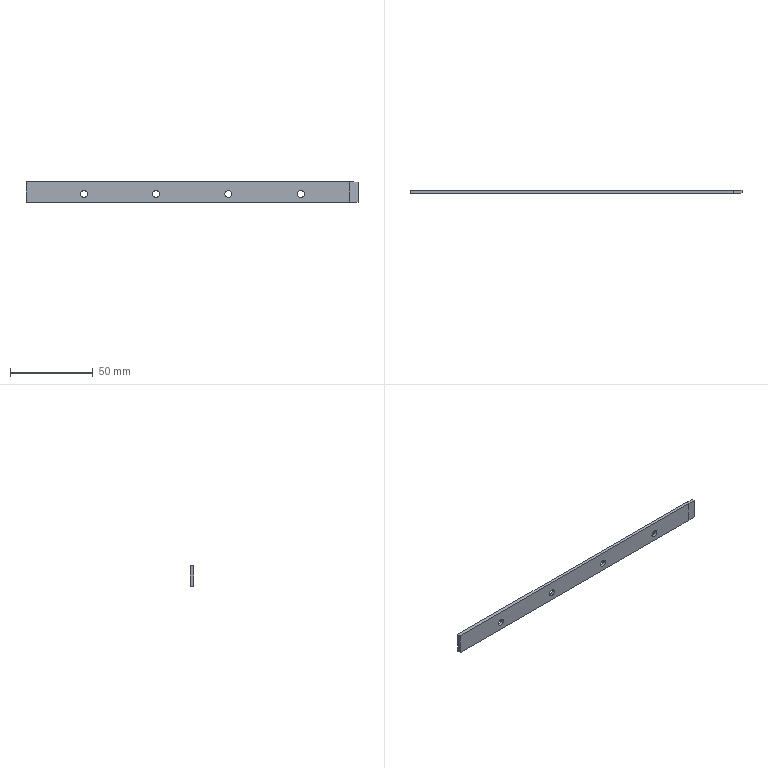Part | NX | 1 solid | 24 faces | box 200 x 2 x 12.5 mm | volume 4873 mm3 | plane 8 | cylinder 8 | cone 8 | commonest cylinder face diameters 4.2 x8
STEP:
#1=CARTESIAN_POINT('',(-140.,215.4,-65.8));
#2=VERTEX_POINT('',#1);
#3=CARTESIAN_POINT('',(-140.,215.4,-53.3));
#4=VERTEX_POINT('',#3);
#5=CARTESIAN_POINT('',(-140.,215.4,-59.293));
#6=DIRECTION('',(0.,0.,1.));
#7=VECTOR('',#6,1000.);
#8=LINE('',#5,#7);
#9=EDGE_CURVE('',#2,#4,#8,.T.);
#10=ORIENTED_EDGE('',*,*,#9,.T.);
#11=CARTESIAN_POINT('',(-140.,217.4,-53.3));
#12=VERTEX_POINT('',#11);
#13=CARTESIAN_POINT('',(-140.,215.4,-53.3));
#14=DIRECTION('',(0.,1.,0.));
#15=VECTOR('',#14,1000.);
#16=LINE('',#13,#15);
#17=EDGE_CURVE('',#4,#12,#16,.T.);
#18=ORIENTED_EDGE('',*,*,#17,.T.);
#19=CARTESIAN_POINT('',(-140.,217.4,-65.8));
#20=VERTEX_POINT('',#19);
#21=CARTESIAN_POINT('',(-140.,217.4,-59.293));
#22=DIRECTION('',(0.,0.,1.));
#23=VECTOR('',#22,1000.);
#24=LINE('',#21,#23);
#25=EDGE_CURVE('',#20,#12,#24,.T.);
#26=ORIENTED_EDGE('',*,*,#25,.F.);
#27=CARTESIAN_POINT('',(-140.,215.4,-65.8));
#28=DIRECTION('',(0.,1.,0.));
#29=VECTOR('',#28,1000.);
#30=LINE('',#27,#29);
#31=EDGE_CURVE('',#2,#20,#30,.T.);
#32=ORIENTED_EDGE('',*,*,#31,.F.);
#33=EDGE_LOOP('',(#10,#18,#26,#32));
#34=FACE_BOUND('',#33,.T.);
#35=CARTESIAN_POINT('',(-140.,215.4,-55.8));
#36=DIRECTION('',(-1.,0.,0.));
#37=DIRECTION('',(0.,0.,1.));
#38=AXIS2_PLACEMENT_3D('',#35,#36,#37);
#39=PLANE('',#38);
#40=ADVANCED_FACE('',(#34),#39,.T.);
#41=CARTESIAN_POINT('',(55.,217.4,-53.3));
#42=VERTEX_POINT('',#41);
#43=CARTESIAN_POINT('',(55.,215.4,-53.3));
#44=VERTEX_POINT('',#43);
#45=CARTESIAN_POINT('',(55.,216.4,-53.3));
#46=DIRECTION('',(0.,-1.,0.));
#47=VECTOR('',#46,1000.);
#48=LINE('',#45,#47);
#49=EDGE_CURVE('',#42,#44,#48,.T.);
#50=ORIENTED_EDGE('',*,*,#49,.F.);
#51=CARTESIAN_POINT('',(-59.483,217.4,-53.3));
#52=DIRECTION('',(1.,0.,0.));
#53=VECTOR('',#52,1000.);
#54=LINE('',#51,#53);
#55=EDGE_CURVE('',#12,#42,#54,.T.);
#56=ORIENTED_EDGE('',*,*,#55,.F.);
#57=ORIENTED_EDGE('',*,*,#17,.F.);
#58=CARTESIAN_POINT('',(-59.483,215.4,-53.3));
#59=DIRECTION('',(1.,0.,0.));
#60=VECTOR('',#59,1000.);
#61=LINE('',#58,#60);
#62=EDGE_CURVE('',#4,#44,#61,.T.);
#63=ORIENTED_EDGE('',*,*,#62,.T.);
#64=EDGE_LOOP('',(#50,#56,#57,#63));
#65=FACE_BOUND('',#64,.T.);
#66=CARTESIAN_POINT('',(60.,215.4,-53.3));
#67=DIRECTION('',(0.,0.,1.));
#68=DIRECTION('',(1.,0.,0.));
#69=AXIS2_PLACEMENT_3D('',#66,#67,#68);
#70=PLANE('',#69);
#71=ADVANCED_FACE('',(#65),#70,.T.);
#72=CARTESIAN_POINT('',(60.,215.837,-53.737));
#73=VERTEX_POINT('',#72);
#74=CARTESIAN_POINT('',(60.,215.837,-65.8));
#75=VERTEX_POINT('',#74);
#76=CARTESIAN_POINT('',(60.,215.837,-59.55));
#77=DIRECTION('',(0.,0.,-1.));
#78=VECTOR('',#77,1000.);
#79=LINE('',#76,#78);
#80=EDGE_CURVE('',#73,#75,#79,.T.);
#81=ORIENTED_EDGE('',*,*,#80,.T.);
#82=CARTESIAN_POINT('',(60.,217.4,-65.8));
#83=VERTEX_POINT('',#82);
#84=CARTESIAN_POINT('',(60.,215.4,-65.8));
#85=DIRECTION('',(0.,1.,0.));
#86=VECTOR('',#85,1000.);
#87=LINE('',#84,#86);
#88=EDGE_CURVE('',#75,#83,#87,.T.);
#89=ORIENTED_EDGE('',*,*,#88,.T.);
#90=CARTESIAN_POINT('',(60.,217.4,-53.737));
#91=VERTEX_POINT('',#90);
#92=CARTESIAN_POINT('',(60.,217.4,-59.293));
#93=DIRECTION('',(0.,0.,-1.));
#94=VECTOR('',#93,1000.);
#95=LINE('',#92,#94);
#96=EDGE_CURVE('',#91,#83,#95,.T.);
#97=ORIENTED_EDGE('',*,*,#96,.F.);
#98=CARTESIAN_POINT('',(60.,216.4,-53.737));
#99=DIRECTION('',(0.,-1.,0.));
#100=VECTOR('',#99,1000.);
#101=LINE('',#98,#100);
#102=EDGE_CURVE('',#91,#73,#101,.T.);
#103=ORIENTED_EDGE('',*,*,#102,.T.);
#104=EDGE_LOOP('',(#81,#89,#97,#103));
#105=FACE_BOUND('',#104,.T.);
#106=CARTESIAN_POINT('',(60.,215.4,-65.8));
#107=DIRECTION('',(1.,0.,0.));
#108=DIRECTION('',(0.,-1.,0.));
#109=AXIS2_PLACEMENT_3D('',#106,#107,#108);
#110=PLANE('',#109);
#111=ADVANCED_FACE('',(#105),#110,.T.);
#112=CARTESIAN_POINT('',(55.,215.4,-65.8));
#113=VERTEX_POINT('',#112);
#114=CARTESIAN_POINT('',(60.,215.4,-65.8));
#115=DIRECTION('',(-1.,0.,0.));
#116=VECTOR('',#115,1000.);
#117=LINE('',#114,#116);
#118=EDGE_CURVE('',#113,#2,#117,.T.);
#119=ORIENTED_EDGE('',*,*,#118,.T.);
#120=ORIENTED_EDGE('',*,*,#31,.T.);
#121=CARTESIAN_POINT('',(60.,217.4,-65.8));
#122=DIRECTION('',(-1.,0.,0.));
#123=VECTOR('',#122,1000.);
#124=LINE('',#121,#123);
#125=EDGE_CURVE('',#83,#20,#124,.T.);
#126=ORIENTED_EDGE('',*,*,#125,.F.);
#127=ORIENTED_EDGE('',*,*,#88,.F.);
#128=CARTESIAN_POINT('',(-59.483,205.384,-65.8));
#129=DIRECTION('',(-0.9962,-0.08716,0.));
#130=VECTOR('',#129,1000.);
#131=LINE('',#128,#130);
#132=EDGE_CURVE('',#75,#113,#131,.T.);
#133=ORIENTED_EDGE('',*,*,#132,.T.);
#134=EDGE_LOOP('',(#119,#120,#126,#127,#133));
#135=FACE_BOUND('',#134,.T.);
#136=CARTESIAN_POINT('',(-140.,215.4,-65.8));
#137=DIRECTION('',(0.,0.,-1.));
#138=DIRECTION('',(0.,-1.,0.));
#139=AXIS2_PLACEMENT_3D('',#136,#137,#138);
#140=PLANE('',#139);
#141=ADVANCED_FACE('',(#135),#140,.T.);
#142=ORIENTED_EDGE('',*,*,#49,.T.);
#143=CARTESIAN_POINT('',(-59.483,205.384,-43.284));
#144=DIRECTION('',(-0.9924,-0.08683,0.08683));
#145=VECTOR('',#144,1000.);
#146=LINE('',#143,#145);
#147=EDGE_CURVE('',#73,#44,#146,.T.);
#148=ORIENTED_EDGE('',*,*,#147,.F.);
#149=ORIENTED_EDGE('',*,*,#102,.F.);
#150=CARTESIAN_POINT('',(-59.483,217.4,-43.284));
#151=DIRECTION('',(0.9962,0.,-0.08716));
#152=VECTOR('',#151,1000.);
#153=LINE('',#150,#152);
#154=EDGE_CURVE('',#42,#91,#153,.T.);
#155=ORIENTED_EDGE('',*,*,#154,.F.);
#156=EDGE_LOOP('',(#142,#148,#149,#155));
#157=FACE_BOUND('',#156,.T.);
#158=CARTESIAN_POINT('',(57.5,216.4,-53.519));
#159=DIRECTION('',(-0.08716,0.,-0.9962));
#160=DIRECTION('',(-0.9962,0.,0.08716));
#161=AXIS2_PLACEMENT_3D('',#158,#159,#160);
#162=PLANE('',#161);
#163=ADVANCED_FACE('',(#157),#162,.F.);
#164=ORIENTED_EDGE('',*,*,#96,.T.);
#165=ORIENTED_EDGE('',*,*,#125,.T.);
#166=ORIENTED_EDGE('',*,*,#25,.T.);
#167=ORIENTED_EDGE('',*,*,#55,.T.);
#168=ORIENTED_EDGE('',*,*,#154,.T.);
#169=EDGE_LOOP('',(#164,#165,#166,#167,#168));
#170=FACE_BOUND('',#169,.T.);
#171=CARTESIAN_POINT('',(27.925,217.4,-60.8));
#172=VERTEX_POINT('',#171);
#173=CARTESIAN_POINT('',(23.325,217.4,-60.8));
#174=VERTEX_POINT('',#173);
#175=CARTESIAN_POINT('',(25.625,217.4,-60.8));
#176=DIRECTION('',(0.,1.,0.));
#177=DIRECTION('',(-1.,0.,0.));
#178=AXIS2_PLACEMENT_3D('',#175,#176,#177);
#179=CIRCLE('',#178,2.3);
#180=EDGE_CURVE('',#172,#174,#179,.T.);
#181=ORIENTED_EDGE('',*,*,#180,.F.);
#182=CARTESIAN_POINT('',(25.625,217.4,-60.8));
#183=DIRECTION('',(0.,1.,0.));
#184=DIRECTION('',(-1.,0.,0.));
#185=AXIS2_PLACEMENT_3D('',#182,#183,#184);
#186=CIRCLE('',#185,2.3);
#187=EDGE_CURVE('',#174,#172,#186,.T.);
#188=ORIENTED_EDGE('',*,*,#187,.F.);
#189=EDGE_LOOP('',(#181,#188));
#190=FACE_BOUND('',#189,.T.);
#191=CARTESIAN_POINT('',(-107.364,217.4,-60.8));
#192=VERTEX_POINT('',#191);
#193=CARTESIAN_POINT('',(-102.764,217.4,-60.8));
#194=VERTEX_POINT('',#193);
#195=CARTESIAN_POINT('',(-105.064,217.4,-60.8));
#196=DIRECTION('',(0.,1.,0.));
#197=DIRECTION('',(-1.,0.,0.));
#198=AXIS2_PLACEMENT_3D('',#195,#196,#197);
#199=CIRCLE('',#198,2.3);
#200=EDGE_CURVE('',#192,#194,#199,.T.);
#201=ORIENTED_EDGE('',*,*,#200,.F.);
#202=CARTESIAN_POINT('',(-105.064,217.4,-60.8));
#203=DIRECTION('',(0.,1.,0.));
#204=DIRECTION('',(-1.,0.,0.));
#205=AXIS2_PLACEMENT_3D('',#202,#203,#204);
#206=CIRCLE('',#205,2.3);
#207=EDGE_CURVE('',#194,#192,#206,.T.);
#208=ORIENTED_EDGE('',*,*,#207,.F.);
#209=EDGE_LOOP('',(#201,#208));
#210=FACE_BOUND('',#209,.T.);
#211=CARTESIAN_POINT('',(-20.425,217.4,-60.8));
#212=VERTEX_POINT('',#211);
#213=CARTESIAN_POINT('',(-15.825,217.4,-60.8));
#214=VERTEX_POINT('',#213);
#215=CARTESIAN_POINT('',(-18.125,217.4,-60.8));
#216=DIRECTION('',(0.,1.,0.));
#217=DIRECTION('',(-1.,0.,0.));
#218=AXIS2_PLACEMENT_3D('',#215,#216,#217);
#219=CIRCLE('',#218,2.3);
#220=EDGE_CURVE('',#212,#214,#219,.T.);
#221=ORIENTED_EDGE('',*,*,#220,.F.);
#222=CARTESIAN_POINT('',(-18.125,217.4,-60.8));
#223=DIRECTION('',(0.,1.,0.));
#224=DIRECTION('',(-1.,0.,0.));
#225=AXIS2_PLACEMENT_3D('',#222,#223,#224);
#226=CIRCLE('',#225,2.3);
#227=EDGE_CURVE('',#214,#212,#226,.T.);
#228=ORIENTED_EDGE('',*,*,#227,.F.);
#229=EDGE_LOOP('',(#221,#228));
#230=FACE_BOUND('',#229,.T.);
#231=CARTESIAN_POINT('',(-59.388,217.4,-60.8));
#232=VERTEX_POINT('',#231);
#233=CARTESIAN_POINT('',(-63.988,217.4,-60.8));
#234=VERTEX_POINT('',#233);
#235=CARTESIAN_POINT('',(-61.688,217.4,-60.8));
#236=DIRECTION('',(0.,1.,0.));
#237=DIRECTION('',(-1.,0.,0.));
#238=AXIS2_PLACEMENT_3D('',#235,#236,#237);
#239=CIRCLE('',#238,2.3);
#240=EDGE_CURVE('',#232,#234,#239,.T.);
#241=ORIENTED_EDGE('',*,*,#240,.F.);
#242=CARTESIAN_POINT('',(-61.688,217.4,-60.8));
#243=DIRECTION('',(0.,1.,0.));
#244=DIRECTION('',(-1.,0.,0.));
#245=AXIS2_PLACEMENT_3D('',#242,#243,#244);
#246=CIRCLE('',#245,2.3);
#247=EDGE_CURVE('',#234,#232,#246,.T.);
#248=ORIENTED_EDGE('',*,*,#247,.F.);
#249=EDGE_LOOP('',(#241,#248));
#250=FACE_BOUND('',#249,.T.);
#251=CARTESIAN_POINT('',(-59.483,217.4,-59.293));
#252=DIRECTION('',(0.,1.,0.));
#253=DIRECTION('',(1.,0.,0.));
#254=AXIS2_PLACEMENT_3D('',#251,#252,#253);
#255=PLANE('',#254);
#256=ADVANCED_FACE('',(#170,#190,#210,#230,#250),#255,.T.);
#257=CARTESIAN_POINT('',(-20.225,215.4,-60.8));
#258=VERTEX_POINT('',#257);
#259=CARTESIAN_POINT('',(-16.025,215.4,-60.8));
#260=VERTEX_POINT('',#259);
#261=CARTESIAN_POINT('',(-18.125,215.4,-60.8));
#262=DIRECTION('',(0.,1.,0.));
#263=DIRECTION('',(-1.,0.,0.));
#264=AXIS2_PLACEMENT_3D('',#261,#262,#263);
#265=CIRCLE('',#264,2.1);
#266=EDGE_CURVE('',#258,#260,#265,.T.);
#267=ORIENTED_EDGE('',*,*,#266,.F.);
#268=CARTESIAN_POINT('',(-20.225,217.2,-60.8));
#269=VERTEX_POINT('',#268);
#270=CARTESIAN_POINT('',(-20.225,217.4,-60.8));
#271=DIRECTION('',(0.,1.,0.));
#272=VECTOR('',#271,1000.);
#273=LINE('',#270,#272);
#274=EDGE_CURVE('',#269,#258,#273,.F.);
#275=ORIENTED_EDGE('',*,*,#274,.F.);
#276=CARTESIAN_POINT('',(-16.025,217.2,-60.8));
#277=VERTEX_POINT('',#276);
#278=CARTESIAN_POINT('',(-18.125,217.2,-60.8));
#279=DIRECTION('',(0.,1.,0.));
#280=DIRECTION('',(-1.,0.,0.));
#281=AXIS2_PLACEMENT_3D('',#278,#279,#280);
#282=CIRCLE('',#281,2.1);
#283=EDGE_CURVE('',#269,#277,#282,.T.);
#284=ORIENTED_EDGE('',*,*,#283,.T.);
#285=CARTESIAN_POINT('',(-16.025,217.4,-60.8));
#286=DIRECTION('',(0.,1.,0.));
#287=VECTOR('',#286,1000.);
#288=LINE('',#285,#287);
#289=EDGE_CURVE('',#277,#260,#288,.F.);
#290=ORIENTED_EDGE('',*,*,#289,.T.);
#291=EDGE_LOOP('',(#267,#275,#284,#290));
#292=FACE_BOUND('',#291,.T.);
#293=CARTESIAN_POINT('',(-18.125,217.4,-60.8));
#294=DIRECTION('',(0.,1.,0.));
#295=DIRECTION('',(-1.,0.,0.));
#296=AXIS2_PLACEMENT_3D('',#293,#294,#295);
#297=CYLINDRICAL_SURFACE('',#296,2.1);
#298=ADVANCED_FACE('',(#292),#297,.F.);
#299=ORIENTED_EDGE('',*,*,#220,.T.);
#300=CARTESIAN_POINT('',(-16.025,217.2,-60.8));
#301=DIRECTION('',(0.7071,0.7071,0.));
#302=VECTOR('',#301,1000.);
#303=LINE('',#300,#302);
#304=EDGE_CURVE('',#277,#214,#303,.T.);
#305=ORIENTED_EDGE('',*,*,#304,.F.);
#306=ORIENTED_EDGE('',*,*,#283,.F.);
#307=CARTESIAN_POINT('',(-20.225,217.2,-60.8));
#308=DIRECTION('',(-0.7071,0.7071,0.));
#309=VECTOR('',#308,1000.);
#310=LINE('',#307,#309);
#311=EDGE_CURVE('',#269,#212,#310,.T.);
#312=ORIENTED_EDGE('',*,*,#311,.T.);
#313=EDGE_LOOP('',(#299,#305,#306,#312));
#314=FACE_BOUND('',#313,.T.);
#315=CARTESIAN_POINT('',(-18.125,217.2,-60.8));
#316=DIRECTION('',(0.,1.,0.));
#317=DIRECTION('',(1.,0.,0.));
#318=AXIS2_PLACEMENT_3D('',#315,#316,#317);
#319=CONICAL_SURFACE('',#318,2.1,0.7854);
#320=ADVANCED_FACE('',(#314),#319,.F.);
#321=CARTESIAN_POINT('',(27.725,215.4,-60.8));
#322=VERTEX_POINT('',#321);
#323=CARTESIAN_POINT('',(23.525,215.4,-60.8));
#324=VERTEX_POINT('',#323);
#325=CARTESIAN_POINT('',(25.625,215.4,-60.8));
#326=DIRECTION('',(0.,1.,0.));
#327=DIRECTION('',(-1.,0.,0.));
#328=AXIS2_PLACEMENT_3D('',#325,#326,#327);
#329=CIRCLE('',#328,2.1);
#330=EDGE_CURVE('',#322,#324,#329,.T.);
#331=ORIENTED_EDGE('',*,*,#330,.F.);
#332=CARTESIAN_POINT('',(27.725,217.2,-60.8));
#333=VERTEX_POINT('',#332);
#334=CARTESIAN_POINT('',(27.725,217.4,-60.8));
#335=DIRECTION('',(0.,1.,0.));
#336=VECTOR('',#335,1000.);
#337=LINE('',#334,#336);
#338=EDGE_CURVE('',#333,#322,#337,.F.);
#339=ORIENTED_EDGE('',*,*,#338,.F.);
#340=CARTESIAN_POINT('',(23.525,217.2,-60.8));
#341=VERTEX_POINT('',#340);
#342=CARTESIAN_POINT('',(25.625,217.2,-60.8));
#343=DIRECTION('',(0.,1.,0.));
#344=DIRECTION('',(-1.,0.,0.));
#345=AXIS2_PLACEMENT_3D('',#342,#343,#344);
#346=CIRCLE('',#345,2.1);
#347=EDGE_CURVE('',#333,#341,#346,.T.);
#348=ORIENTED_EDGE('',*,*,#347,.T.);
#349=CARTESIAN_POINT('',(23.525,217.4,-60.8));
#350=DIRECTION('',(0.,1.,0.));
#351=VECTOR('',#350,1000.);
#352=LINE('',#349,#351);
#353=EDGE_CURVE('',#341,#324,#352,.F.);
#354=ORIENTED_EDGE('',*,*,#353,.T.);
#355=EDGE_LOOP('',(#331,#339,#348,#354));
#356=FACE_BOUND('',#355,.T.);
#357=CARTESIAN_POINT('',(25.625,217.4,-60.8));
#358=DIRECTION('',(0.,1.,0.));
#359=DIRECTION('',(-1.,0.,0.));
#360=AXIS2_PLACEMENT_3D('',#357,#358,#359);
#361=CYLINDRICAL_SURFACE('',#360,2.1);
#362=ADVANCED_FACE('',(#356),#361,.F.);
#363=ORIENTED_EDGE('',*,*,#347,.F.);
#364=CARTESIAN_POINT('',(27.725,217.2,-60.8));
#365=DIRECTION('',(0.7071,0.7071,0.));
#366=VECTOR('',#365,1000.);
#367=LINE('',#364,#366);
#368=EDGE_CURVE('',#333,#172,#367,.T.);
#369=ORIENTED_EDGE('',*,*,#368,.T.);
#370=ORIENTED_EDGE('',*,*,#180,.T.);
#371=CARTESIAN_POINT('',(23.525,217.2,-60.8));
#372=DIRECTION('',(-0.7071,0.7071,0.));
#373=VECTOR('',#372,1000.);
#374=LINE('',#371,#373);
#375=EDGE_CURVE('',#341,#174,#374,.T.);
#376=ORIENTED_EDGE('',*,*,#375,.F.);
#377=EDGE_LOOP('',(#363,#369,#370,#376));
#378=FACE_BOUND('',#377,.T.);
#379=CARTESIAN_POINT('',(25.625,217.2,-60.8));
#380=DIRECTION('',(0.,1.,0.));
#381=DIRECTION('',(1.,0.,0.));
#382=AXIS2_PLACEMENT_3D('',#379,#380,#381);
#383=CONICAL_SURFACE('',#382,2.1,0.7854);
#384=ADVANCED_FACE('',(#378),#383,.F.);
#385=CARTESIAN_POINT('',(-63.788,217.2,-60.8));
#386=VERTEX_POINT('',#385);
#387=CARTESIAN_POINT('',(-59.588,217.2,-60.8));
#388=VERTEX_POINT('',#387);
#389=CARTESIAN_POINT('',(-61.688,217.2,-60.8));
#390=DIRECTION('',(0.,1.,0.));
#391=DIRECTION('',(-1.,0.,0.));
#392=AXIS2_PLACEMENT_3D('',#389,#390,#391);
#393=CIRCLE('',#392,2.1);
#394=EDGE_CURVE('',#386,#388,#393,.T.);
#395=ORIENTED_EDGE('',*,*,#394,.T.);
#396=CARTESIAN_POINT('',(-59.588,215.4,-60.8));
#397=VERTEX_POINT('',#396);
#398=CARTESIAN_POINT('',(-59.588,217.4,-60.8));
#399=DIRECTION('',(0.,1.,0.));
#400=VECTOR('',#399,1000.);
#401=LINE('',#398,#400);
#402=EDGE_CURVE('',#388,#397,#401,.F.);
#403=ORIENTED_EDGE('',*,*,#402,.T.);
#404=CARTESIAN_POINT('',(-63.788,215.4,-60.8));
#405=VERTEX_POINT('',#404);
#406=CARTESIAN_POINT('',(-61.688,215.4,-60.8));
#407=DIRECTION('',(0.,1.,0.));
#408=DIRECTION('',(-1.,0.,0.));
#409=AXIS2_PLACEMENT_3D('',#406,#407,#408);
#410=CIRCLE('',#409,2.1);
#411=EDGE_CURVE('',#405,#397,#410,.T.);
#412=ORIENTED_EDGE('',*,*,#411,.F.);
#413=CARTESIAN_POINT('',(-63.788,217.4,-60.8));
#414=DIRECTION('',(0.,1.,0.));
#415=VECTOR('',#414,1000.);
#416=LINE('',#413,#415);
#417=EDGE_CURVE('',#386,#405,#416,.F.);
#418=ORIENTED_EDGE('',*,*,#417,.F.);
#419=EDGE_LOOP('',(#395,#403,#412,#418));
#420=FACE_BOUND('',#419,.T.);
#421=CARTESIAN_POINT('',(-61.688,217.4,-60.8));
#422=DIRECTION('',(0.,1.,0.));
#423=DIRECTION('',(-1.,0.,0.));
#424=AXIS2_PLACEMENT_3D('',#421,#422,#423);
#425=CYLINDRICAL_SURFACE('',#424,2.1);
#426=ADVANCED_FACE('',(#420),#425,.F.);
#427=ORIENTED_EDGE('',*,*,#240,.T.);
#428=CARTESIAN_POINT('',(-63.788,217.2,-60.8));
#429=DIRECTION('',(-0.7071,0.7071,0.));
#430=VECTOR('',#429,1000.);
#431=LINE('',#428,#430);
#432=EDGE_CURVE('',#234,#386,#431,.F.);
#433=ORIENTED_EDGE('',*,*,#432,.T.);
#434=CARTESIAN_POINT('',(-61.688,217.2,-60.8));
#435=DIRECTION('',(0.,1.,0.));
#436=DIRECTION('',(-1.,0.,0.));
#437=AXIS2_PLACEMENT_3D('',#434,#435,#436);
#438=CIRCLE('',#437,2.1);
#439=EDGE_CURVE('',#388,#386,#438,.T.);
#440=ORIENTED_EDGE('',*,*,#439,.F.);
#441=CARTESIAN_POINT('',(-59.588,217.2,-60.8));
#442=DIRECTION('',(0.7071,0.7071,0.));
#443=VECTOR('',#442,1000.);
#444=LINE('',#441,#443);
#445=EDGE_CURVE('',#232,#388,#444,.F.);
#446=ORIENTED_EDGE('',*,*,#445,.F.);
#447=EDGE_LOOP('',(#427,#433,#440,#446));
#448=FACE_BOUND('',#447,.T.);
#449=CARTESIAN_POINT('',(-61.688,217.2,-60.8));
#450=DIRECTION('',(0.,1.,0.));
#451=DIRECTION('',(1.,0.,0.));
#452=AXIS2_PLACEMENT_3D('',#449,#450,#451);
#453=CONICAL_SURFACE('',#452,2.1,0.7854);
#454=ADVANCED_FACE('',(#448),#453,.F.);
#455=CARTESIAN_POINT('',(-107.164,217.2,-60.8));
#456=VERTEX_POINT('',#455);
#457=CARTESIAN_POINT('',(-102.964,217.2,-60.8));
#458=VERTEX_POINT('',#457);
#459=CARTESIAN_POINT('',(-105.064,217.2,-60.8));
#460=DIRECTION('',(0.,1.,0.));
#461=DIRECTION('',(-1.,0.,0.));
#462=AXIS2_PLACEMENT_3D('',#459,#460,#461);
#463=CIRCLE('',#462,2.1);
#464=EDGE_CURVE('',#456,#458,#463,.T.);
#465=ORIENTED_EDGE('',*,*,#464,.T.);
#466=CARTESIAN_POINT('',(-102.964,215.4,-60.8));
#467=VERTEX_POINT('',#466);
#468=CARTESIAN_POINT('',(-102.964,217.4,-60.8));
#469=DIRECTION('',(0.,1.,0.));
#470=VECTOR('',#469,1000.);
#471=LINE('',#468,#470);
#472=EDGE_CURVE('',#467,#458,#471,.T.);
#473=ORIENTED_EDGE('',*,*,#472,.F.);
#474=CARTESIAN_POINT('',(-107.164,215.4,-60.8));
#475=VERTEX_POINT('',#474);
#476=CARTESIAN_POINT('',(-105.064,215.4,-60.8));
#477=DIRECTION('',(0.,1.,0.));
#478=DIRECTION('',(-1.,0.,0.));
#479=AXIS2_PLACEMENT_3D('',#476,#477,#478);
#480=CIRCLE('',#479,2.1);
#481=EDGE_CURVE('',#475,#467,#480,.T.);
#482=ORIENTED_EDGE('',*,*,#481,.F.);
#483=CARTESIAN_POINT('',(-107.164,217.4,-60.8));
#484=DIRECTION('',(0.,1.,0.));
#485=VECTOR('',#484,1000.);
#486=LINE('',#483,#485);
#487=EDGE_CURVE('',#475,#456,#486,.T.);
#488=ORIENTED_EDGE('',*,*,#487,.T.);
#489=EDGE_LOOP('',(#465,#473,#482,#488));
#490=FACE_BOUND('',#489,.T.);
#491=CARTESIAN_POINT('',(-105.064,217.4,-60.8));
#492=DIRECTION('',(0.,1.,0.));
#493=DIRECTION('',(-1.,0.,0.));
#494=AXIS2_PLACEMENT_3D('',#491,#492,#493);
#495=CYLINDRICAL_SURFACE('',#494,2.1);
#496=ADVANCED_FACE('',(#490),#495,.F.);
#497=ORIENTED_EDGE('',*,*,#464,.F.);
#498=CARTESIAN_POINT('',(-107.164,217.2,-60.8));
#499=DIRECTION('',(-0.7071,0.7071,0.));
#500=VECTOR('',#499,1000.);
#501=LINE('',#498,#500);
#502=EDGE_CURVE('',#456,#192,#501,.T.);
#503=ORIENTED_EDGE('',*,*,#502,.T.);
#504=ORIENTED_EDGE('',*,*,#200,.T.);
#505=CARTESIAN_POINT('',(-102.964,217.2,-60.8));
#506=DIRECTION('',(0.7071,0.7071,0.));
#507=VECTOR('',#506,1000.);
#508=LINE('',#505,#507);
#509=EDGE_CURVE('',#458,#194,#508,.T.);
#510=ORIENTED_EDGE('',*,*,#509,.F.);
#511=EDGE_LOOP('',(#497,#503,#504,#510));
#512=FACE_BOUND('',#511,.T.);
#513=CARTESIAN_POINT('',(-105.064,217.2,-60.8));
#514=DIRECTION('',(0.,1.,0.));
#515=DIRECTION('',(1.,0.,0.));
#516=AXIS2_PLACEMENT_3D('',#513,#514,#515);
#517=CONICAL_SURFACE('',#516,2.1,0.7854);
#518=ADVANCED_FACE('',(#512),#517,.F.);
#519=CARTESIAN_POINT('',(55.,215.4,-59.55));
#520=DIRECTION('',(0.,0.,-1.));
#521=VECTOR('',#520,1000.);
#522=LINE('',#519,#521);
#523=EDGE_CURVE('',#44,#113,#522,.T.);
#524=ORIENTED_EDGE('',*,*,#523,.T.);
#525=ORIENTED_EDGE('',*,*,#132,.F.);
#526=ORIENTED_EDGE('',*,*,#80,.F.);
#527=ORIENTED_EDGE('',*,*,#147,.T.);
#528=EDGE_LOOP('',(#524,#525,#526,#527));
#529=FACE_BOUND('',#528,.T.);
#530=CARTESIAN_POINT('',(57.5,215.619,-59.55));
#531=DIRECTION('',(-0.08716,0.9962,0.));
#532=DIRECTION('',(0.,0.,1.));
#533=AXIS2_PLACEMENT_3D('',#530,#531,#532);
#534=PLANE('',#533);
#535=ADVANCED_FACE('',(#529),#534,.F.);
#536=ORIENTED_EDGE('',*,*,#523,.F.);
#537=ORIENTED_EDGE('',*,*,#62,.F.);
#538=ORIENTED_EDGE('',*,*,#9,.F.);
#539=ORIENTED_EDGE('',*,*,#118,.F.);
#540=EDGE_LOOP('',(#536,#537,#538,#539));
#541=FACE_BOUND('',#540,.T.);
#542=ORIENTED_EDGE('',*,*,#330,.T.);
#543=CARTESIAN_POINT('',(25.625,215.4,-60.8));
#544=DIRECTION('',(0.,1.,0.));
#545=DIRECTION('',(-1.,0.,0.));
#546=AXIS2_PLACEMENT_3D('',#543,#544,#545);
#547=CIRCLE('',#546,2.1);
#548=EDGE_CURVE('',#324,#322,#547,.T.);
#549=ORIENTED_EDGE('',*,*,#548,.T.);
#550=EDGE_LOOP('',(#542,#549));
#551=FACE_BOUND('',#550,.T.);
#552=ORIENTED_EDGE('',*,*,#411,.T.);
#553=CARTESIAN_POINT('',(-61.688,215.4,-60.8));
#554=DIRECTION('',(0.,1.,0.));
#555=DIRECTION('',(-1.,0.,0.));
#556=AXIS2_PLACEMENT_3D('',#553,#554,#555);
#557=CIRCLE('',#556,2.1);
#558=EDGE_CURVE('',#397,#405,#557,.T.);
#559=ORIENTED_EDGE('',*,*,#558,.T.);
#560=EDGE_LOOP('',(#552,#559));
#561=FACE_BOUND('',#560,.T.);
#562=CARTESIAN_POINT('',(-105.064,215.4,-60.8));
#563=DIRECTION('',(0.,1.,0.));
#564=DIRECTION('',(-1.,0.,0.));
#565=AXIS2_PLACEMENT_3D('',#562,#563,#564);
#566=CIRCLE('',#565,2.1);
#567=EDGE_CURVE('',#467,#475,#566,.T.);
#568=ORIENTED_EDGE('',*,*,#567,.T.);
#569=ORIENTED_EDGE('',*,*,#481,.T.);
#570=EDGE_LOOP('',(#568,#569));
#571=FACE_BOUND('',#570,.T.);
#572=ORIENTED_EDGE('',*,*,#266,.T.);
#573=CARTESIAN_POINT('',(-18.125,215.4,-60.8));
#574=DIRECTION('',(0.,1.,0.));
#575=DIRECTION('',(-1.,0.,0.));
#576=AXIS2_PLACEMENT_3D('',#573,#574,#575);
#577=CIRCLE('',#576,2.1);
#578=EDGE_CURVE('',#260,#258,#577,.T.);
#579=ORIENTED_EDGE('',*,*,#578,.T.);
#580=EDGE_LOOP('',(#572,#579));
#581=FACE_BOUND('',#580,.T.);
#582=CARTESIAN_POINT('',(-59.483,215.4,-59.293));
#583=DIRECTION('',(0.,1.,0.));
#584=DIRECTION('',(1.,0.,0.));
#585=AXIS2_PLACEMENT_3D('',#582,#583,#584);
#586=PLANE('',#585);
#587=ADVANCED_FACE('',(#541,#551,#561,#571,#581),#586,.F.);
#588=ORIENTED_EDGE('',*,*,#274,.T.);
#589=ORIENTED_EDGE('',*,*,#578,.F.);
#590=ORIENTED_EDGE('',*,*,#289,.F.);
#591=CARTESIAN_POINT('',(-18.125,217.2,-60.8));
#592=DIRECTION('',(0.,1.,0.));
#593=DIRECTION('',(-1.,0.,0.));
#594=AXIS2_PLACEMENT_3D('',#591,#592,#593);
#595=CIRCLE('',#594,2.1);
#596=EDGE_CURVE('',#277,#269,#595,.T.);
#597=ORIENTED_EDGE('',*,*,#596,.T.);
#598=EDGE_LOOP('',(#588,#589,#590,#597));
#599=FACE_BOUND('',#598,.T.);
#600=CARTESIAN_POINT('',(-18.125,217.4,-60.8));
#601=DIRECTION('',(0.,1.,0.));
#602=DIRECTION('',(-1.,0.,0.));
#603=AXIS2_PLACEMENT_3D('',#600,#601,#602);
#604=CYLINDRICAL_SURFACE('',#603,2.1);
#605=ADVANCED_FACE('',(#599),#604,.F.);
#606=ORIENTED_EDGE('',*,*,#509,.T.);
#607=ORIENTED_EDGE('',*,*,#207,.T.);
#608=ORIENTED_EDGE('',*,*,#502,.F.);
#609=CARTESIAN_POINT('',(-105.064,217.2,-60.8));
#610=DIRECTION('',(0.,1.,0.));
#611=DIRECTION('',(-1.,0.,0.));
#612=AXIS2_PLACEMENT_3D('',#609,#610,#611);
#613=CIRCLE('',#612,2.1);
#614=EDGE_CURVE('',#458,#456,#613,.T.);
#615=ORIENTED_EDGE('',*,*,#614,.F.);
#616=EDGE_LOOP('',(#606,#607,#608,#615));
#617=FACE_BOUND('',#616,.T.);
#618=CARTESIAN_POINT('',(-105.064,217.2,-60.8));
#619=DIRECTION('',(0.,1.,0.));
#620=DIRECTION('',(1.,0.,0.));
#621=AXIS2_PLACEMENT_3D('',#618,#619,#620);
#622=CONICAL_SURFACE('',#621,2.1,0.7854);
#623=ADVANCED_FACE('',(#617),#622,.F.);
#624=ORIENTED_EDGE('',*,*,#353,.F.);
#625=CARTESIAN_POINT('',(25.625,217.2,-60.8));
#626=DIRECTION('',(0.,1.,0.));
#627=DIRECTION('',(-1.,0.,0.));
#628=AXIS2_PLACEMENT_3D('',#625,#626,#627);
#629=CIRCLE('',#628,2.1);
#630=EDGE_CURVE('',#341,#333,#629,.T.);
#631=ORIENTED_EDGE('',*,*,#630,.T.);
#632=ORIENTED_EDGE('',*,*,#338,.T.);
#633=ORIENTED_EDGE('',*,*,#548,.F.);
#634=EDGE_LOOP('',(#624,#631,#632,#633));
#635=FACE_BOUND('',#634,.T.);
#636=CARTESIAN_POINT('',(25.625,217.4,-60.8));
#637=DIRECTION('',(0.,1.,0.));
#638=DIRECTION('',(-1.,0.,0.));
#639=AXIS2_PLACEMENT_3D('',#636,#637,#638);
#640=CYLINDRICAL_SURFACE('',#639,2.1);
#641=ADVANCED_FACE('',(#635),#640,.F.);
#642=ORIENTED_EDGE('',*,*,#394,.F.);
#643=ORIENTED_EDGE('',*,*,#432,.F.);
#644=ORIENTED_EDGE('',*,*,#247,.T.);
#645=ORIENTED_EDGE('',*,*,#445,.T.);
#646=EDGE_LOOP('',(#642,#643,#644,#645));
#647=FACE_BOUND('',#646,.T.);
#648=CARTESIAN_POINT('',(-61.688,217.2,-60.8));
#649=DIRECTION('',(0.,1.,0.));
#650=DIRECTION('',(1.,0.,0.));
#651=AXIS2_PLACEMENT_3D('',#648,#649,#650);
#652=CONICAL_SURFACE('',#651,2.1,0.7854);
#653=ADVANCED_FACE('',(#647),#652,.F.);
#654=ORIENTED_EDGE('',*,*,#567,.F.);
#655=ORIENTED_EDGE('',*,*,#472,.T.);
#656=ORIENTED_EDGE('',*,*,#614,.T.);
#657=ORIENTED_EDGE('',*,*,#487,.F.);
#658=EDGE_LOOP('',(#654,#655,#656,#657));
#659=FACE_BOUND('',#658,.T.);
#660=CARTESIAN_POINT('',(-105.064,217.4,-60.8));
#661=DIRECTION('',(0.,1.,0.));
#662=DIRECTION('',(-1.,0.,0.));
#663=AXIS2_PLACEMENT_3D('',#660,#661,#662);
#664=CYLINDRICAL_SURFACE('',#663,2.1);
#665=ADVANCED_FACE('',(#659),#664,.F.);
#666=ORIENTED_EDGE('',*,*,#368,.F.);
#667=ORIENTED_EDGE('',*,*,#630,.F.);
#668=ORIENTED_EDGE('',*,*,#375,.T.);
#669=ORIENTED_EDGE('',*,*,#187,.T.);
#670=EDGE_LOOP('',(#666,#667,#668,#669));
#671=FACE_BOUND('',#670,.T.);
#672=CARTESIAN_POINT('',(25.625,217.2,-60.8));
#673=DIRECTION('',(0.,1.,0.));
#674=DIRECTION('',(1.,0.,0.));
#675=AXIS2_PLACEMENT_3D('',#672,#673,#674);
#676=CONICAL_SURFACE('',#675,2.1,0.7854);
#677=ADVANCED_FACE('',(#671),#676,.F.);
#678=ORIENTED_EDGE('',*,*,#417,.T.);
#679=ORIENTED_EDGE('',*,*,#558,.F.);
#680=ORIENTED_EDGE('',*,*,#402,.F.);
#681=ORIENTED_EDGE('',*,*,#439,.T.);
#682=EDGE_LOOP('',(#678,#679,#680,#681));
#683=FACE_BOUND('',#682,.T.);
#684=CARTESIAN_POINT('',(-61.688,217.4,-60.8));
#685=DIRECTION('',(0.,1.,0.));
#686=DIRECTION('',(-1.,0.,0.));
#687=AXIS2_PLACEMENT_3D('',#684,#685,#686);
#688=CYLINDRICAL_SURFACE('',#687,2.1);
#689=ADVANCED_FACE('',(#683),#688,.F.);
#690=ORIENTED_EDGE('',*,*,#304,.T.);
#691=ORIENTED_EDGE('',*,*,#227,.T.);
#692=ORIENTED_EDGE('',*,*,#311,.F.);
#693=ORIENTED_EDGE('',*,*,#596,.F.);
#694=EDGE_LOOP('',(#690,#691,#692,#693));
#695=FACE_BOUND('',#694,.T.);
#696=CARTESIAN_POINT('',(-18.125,217.2,-60.8));
#697=DIRECTION('',(0.,1.,0.));
#698=DIRECTION('',(1.,0.,0.));
#699=AXIS2_PLACEMENT_3D('',#696,#697,#698);
#700=CONICAL_SURFACE('',#699,2.1,0.7854);
#701=ADVANCED_FACE('',(#695),#700,.F.);
#702=CLOSED_SHELL('',(#40,#71,#111,#141,#163,#256,#298,#320,#362,#384,#426,#454,#496,#518,#535,#587,#605,#623,#641,#653,#665,#677,#689,#701));
#703=MANIFOLD_SOLID_BREP('',#702);
#704=(LENGTH_UNIT()NAMED_UNIT(*)SI_UNIT(.MILLI.,.METRE.));
#705=UNCERTAINTY_MEASURE_WITH_UNIT(LENGTH_MEASURE(0.00001),#704,'','');
#706=(NAMED_UNIT(*)PLANE_ANGLE_UNIT()SI_UNIT($,.RADIAN.));
#707=(NAMED_UNIT(*)SI_UNIT($,.STERADIAN.)SOLID_ANGLE_UNIT());
#708=(GEOMETRIC_REPRESENTATION_CONTEXT(3)GLOBAL_UNCERTAINTY_ASSIGNED_CONTEXT((#705))GLOBAL_UNIT_ASSIGNED_CONTEXT((#704,#706,#707))REPRESENTATION_CONTEXT('',''));
#709=ADVANCED_BREP_SHAPE_REPRESENTATION('',(#703),#708);